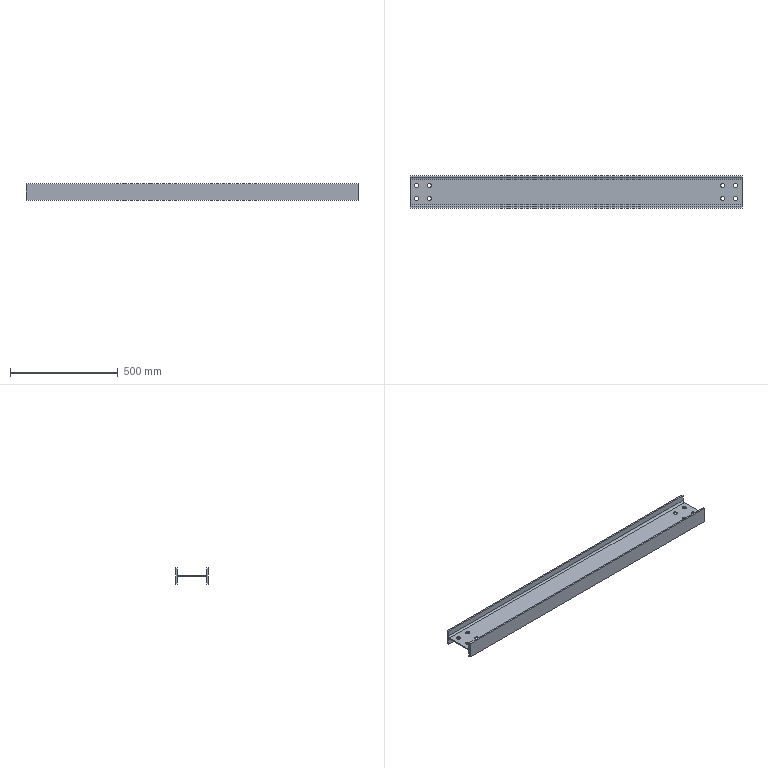Part | STEP file | 计量辅梁5主体_Default<As Machined> | 1 solid | 34 faces | box 1540 x 150 x 75 mm | volume 2737463 mm3 | cylinder 20 | plane 14 | commonest cylinder face diameters 19 x16 16 x4